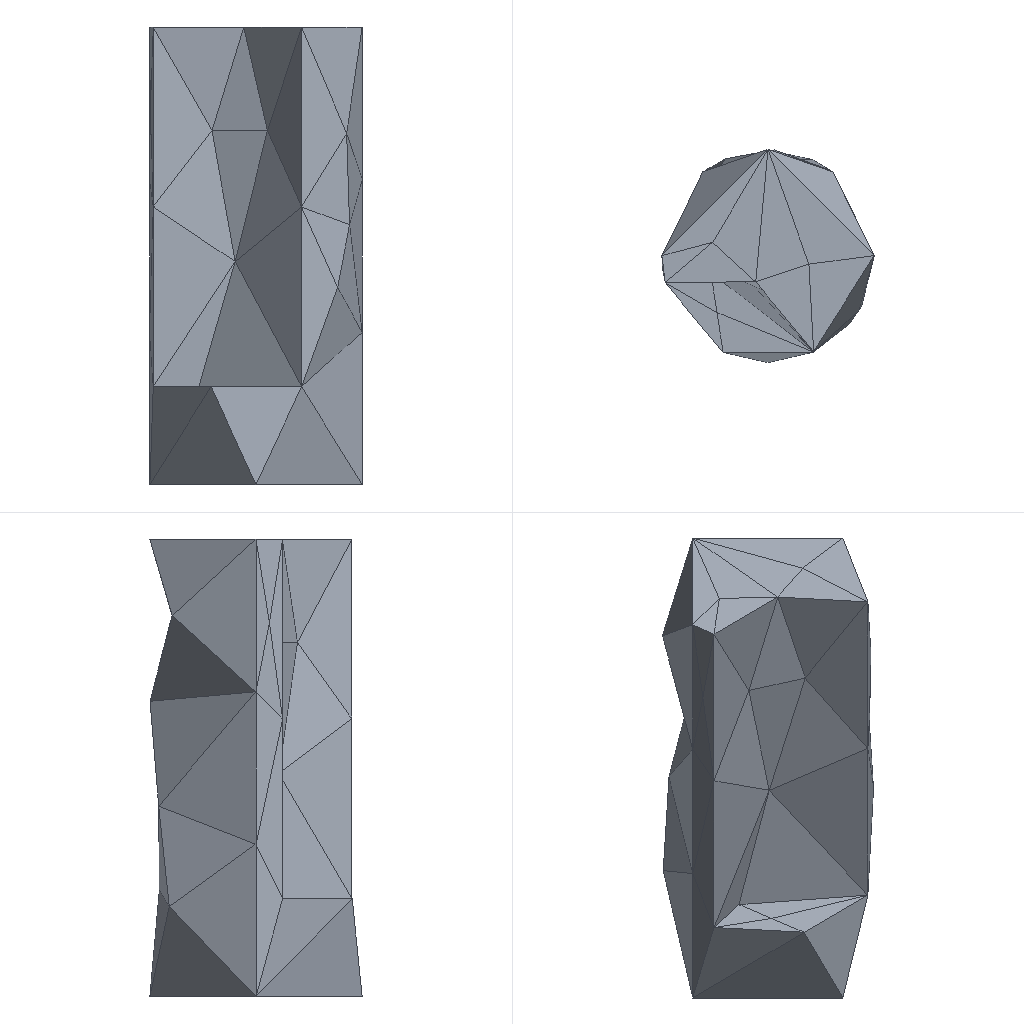Simulation study | ansys mapdl
Set-up summary:
category,name,step,type,value,unit,region
solver,ansys_mapdl
units,mm-N-s-tonne (MPa),,inferred,E=210000 density=
analysis,model,,static
mesh,nodes,,,205
mesh,elements,,,90
element_type,SOLID187,,,90
material,mat 1,,E,210000
material,mat 1,,nu,0.3
load,,model,body load temp,,,all
load,,model,force,"1000 [dir=(0, 0, -1) n=49]",,node list
bc,,model,fixed,"[dofs=UX,UY,UZ n=230]",,node list
Ansys APDL input file, long lists of numbers shortened:
/COM,ANSYS RELEASE 2026 R1           BUILD 26.1      UP20260202       09:11:27
/PREP7
/NOPR
/TITLE,2
ANTYPE, 0
*IF,_CDRDOFF,EQ,1,THEN     !if solid model was read in
_CDRDOFF=             !reset flag, numoffs already performed
*ELSE              !offset database for the following FE model
NUMOFF,NODE,      205
NUMOFF,ELEM,       90
NUMOFF,MAT ,        1
NUMOFF,TYPE,        1
*ENDIF
*SET,_RETURN ,  0.
*SET,_STATUS ,  0.
*SET,_UIQR   ,  49.
*SET,__FLOATPARAMETER__,  205.
DOF,DELETE
ETBLOCK,        1,        1
(2i9,19a9)
        1      187        0        0        0        0        0        0        0        0        0        0        0        0        0        0        0        0        0        0        0
       -1
NBLOCK,6,SOLID,       205,       205
(3i9,6e21.13e3)
        1        0        0 2.7000000000000E+001-1.1500000000000E+001 5.0000000000000E+000
! (204 more lines like these left out)
N,UNBL,LOC,       -1,
EBLOCK,19,SOLID,        90,        90
(19i10)
         1         1         1         1         0         0         0         0        10         0         1       124        34        73       110       116        74       114       149
! (179 more lines like these left out)
        -1
MPTEMP,UNBL, 1, 1,  0.    ,
MPDATA,UNBL, 1,EX  ,       1, 1,  210000.000    ,
MPTEMP,UNBL, 1, 1,  0.    ,
MPDATA,UNBL, 1,NUXY,       1, 1, 0.3    ,
MPTEMP,UNBL, 1, 1,  0.    ,
MPDATA,UNBL, 1,PRXY,       1, 1, 0.3    ,
EXTOPT,ATTR,      0,      0,      0
EXTOPT,ESIZE,  0,  0.
EXTOPT,ACLEAR,      0
TREF,  0.
IRLF,  0
BFUNIF,TEMP,_TINY
ACEL,  0.    ,  0.    ,  0.
OMEGA,  0.    ,  0.    ,  0.
DOMEGA,  0.    ,  0.    ,  0.
CGLOC,  0.    ,  0.    ,  0.
CGOMEGA,  0.    ,  0.    ,  0.
DCGOMG,  0.    ,  0.    ,  0.
KUSE,     0
TIME,  0.
ALPHAD,  0.
BETAD,  0.
DMPRAT,  0.
DMPSTR,  0.
CRPLIM, 0.1    ,   0
CRPLIM,  0.    ,   1
NCNV,     0, 1.000000000E+12,     0,  0.    ,  0.
NEQIT,     0
ERESX,DEFA
DBLOCK,       230
(i9,a6,2(pg16.9))
        1  UX    0.00000000      0.00000000
! (229 more lines like these left out)
       -1
FBLOCK,        49
(i9,a6,2(pg16.9))
       19  FZ   -20.4081633      0.00000000
! (48 more lines like these left out)
       -1
/GO
FINISH
Results summary:
result,analysis_type_db,,,static,unstated
result,n_sets,,,1,unstated
result,load_steps[0].set,load_step=1,,1,unstated
result,load_steps[0].substep,load_step=1,,1,unstated
result,load_steps[0].time,load_step=1,,1,unstated
result,load_steps[0].freq,load_step=1,,1,unstated
result,load_steps[0].max_usum,load_step=1,,0.001564,unstated
result,load_steps[0].max_seqv,load_step=1,,24.837,unstated
result,load_steps[0].reaction_sum.FX,load_step=1,,-1.51212e-11,unstated
result,load_steps[0].reaction_sum.FY,load_step=1,,-3.48876e-12,unstated
result,load_steps[0].reaction_sum.FZ,load_step=1,,1000,unstated
result,load_steps[0].reaction_sum.MX,load_step=1,,0,unstated
result,load_steps[0].reaction_sum.MY,load_step=1,,0,unstated
result,load_steps[0].reaction_sum.MZ,load_step=1,,0,unstated
result,convergence,,,results present for all listed sets,unstated